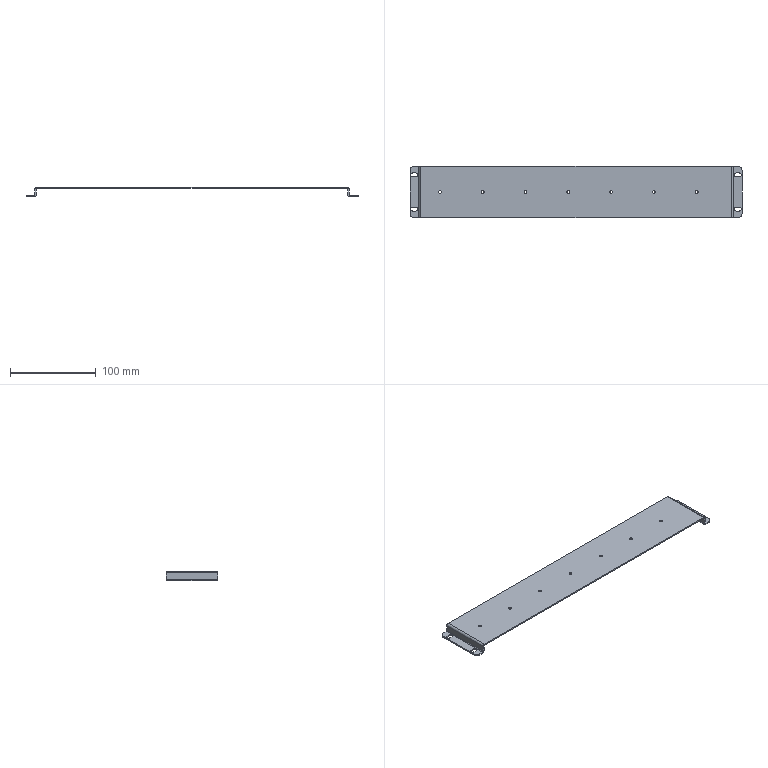Part | STEP file | 03-34 cable tray mounting plate (Default) | 1 solid | 76 faces | box 388 x 60 x 11.5 mm | volume 36165 mm3 | cylinder 38 | plane 38 | commonest cylinder face diameters 3.3 x14 4.5 x12 1.473 x4 4.473 x4 10 x4